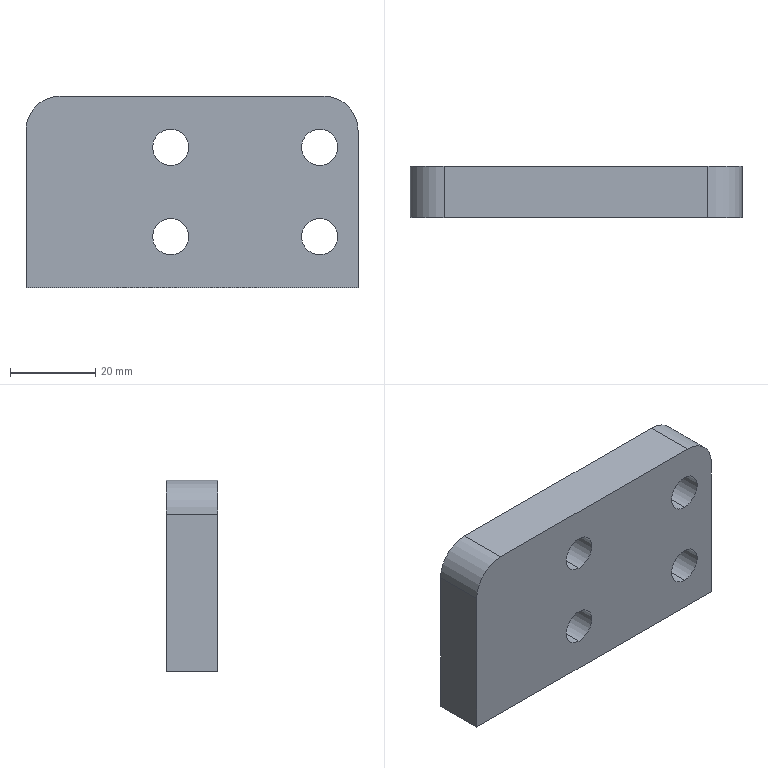Part | SolidWorks | features BaseBody 1 | 1 solid | 36 faces | box 78 x 12 x 45 mm | volume 35458 mm3 | cone 16 | cylinder 14 | plane 6 | commonest cylinder face diameters 8.5 x12 16 x2
STEP:
#1=CARTESIAN_POINT('',(30.,11.225,-14.75));
#2=VERTEX_POINT('',#1);
#3=CARTESIAN_POINT('',(30.,11.225,-6.25));
#4=VERTEX_POINT('',#3);
#5=CARTESIAN_POINT('',(30.,11.225,-10.5));
#6=DIRECTION('',(0.,1.,0.));
#7=DIRECTION('',(0.,0.,1.));
#8=AXIS2_PLACEMENT_3D('',#5,#6,#7);
#9=CIRCLE('',#8,4.25);
#10=EDGE_CURVE('',#2,#4,#9,.T.);
#11=ORIENTED_EDGE('',*,*,#10,.F.);
#12=CARTESIAN_POINT('',(30.,12.,-15.525));
#13=VERTEX_POINT('',#12);
#14=CARTESIAN_POINT('',(30.,12.,-15.525));
#15=DIRECTION('',(0.,0.7071,-0.7071));
#16=VECTOR('',#15,1000.);
#17=LINE('',#14,#16);
#18=EDGE_CURVE('',#2,#13,#17,.T.);
#19=ORIENTED_EDGE('',*,*,#18,.T.);
#20=CARTESIAN_POINT('',(30.,12.,-5.475));
#21=VERTEX_POINT('',#20);
#22=CARTESIAN_POINT('',(30.,12.,-10.5));
#23=DIRECTION('',(0.,1.,0.));
#24=DIRECTION('',(0.,0.,1.));
#25=AXIS2_PLACEMENT_3D('',#22,#23,#24);
#26=CIRCLE('',#25,5.025);
#27=EDGE_CURVE('',#13,#21,#26,.T.);
#28=ORIENTED_EDGE('',*,*,#27,.T.);
#29=CARTESIAN_POINT('',(30.,12.,-5.475));
#30=DIRECTION('',(0.,0.7071,0.7071));
#31=VECTOR('',#30,1000.);
#32=LINE('',#29,#31);
#33=EDGE_CURVE('',#4,#21,#32,.T.);
#34=ORIENTED_EDGE('',*,*,#33,.F.);
#35=EDGE_LOOP('',(#11,#19,#28,#34));
#36=FACE_OUTER_BOUND('',#35,.T.);
#37=CARTESIAN_POINT('',(30.,12.,-10.5));
#38=DIRECTION('',(0.,1.,0.));
#39=DIRECTION('',(0.,0.,1.));
#40=AXIS2_PLACEMENT_3D('',#37,#38,#39);
#41=CONICAL_SURFACE('',#40,5.025,0.7854);
#42=ADVANCED_FACE('',(#36),#41,.F.);
#43=CARTESIAN_POINT('',(30.,0.,-14.75));
#44=VERTEX_POINT('',#43);
#45=CARTESIAN_POINT('',(30.,0.,-6.25));
#46=VERTEX_POINT('',#45);
#47=CARTESIAN_POINT('',(30.,0.,-10.5));
#48=DIRECTION('',(0.,1.,0.));
#49=DIRECTION('',(0.,0.,1.));
#50=AXIS2_PLACEMENT_3D('',#47,#48,#49);
#51=CIRCLE('',#50,4.25);
#52=EDGE_CURVE('',#44,#46,#51,.T.);
#53=ORIENTED_EDGE('',*,*,#52,.F.);
#54=CARTESIAN_POINT('',(30.,12.,-14.75));
#55=DIRECTION('',(0.,1.,0.));
#56=VECTOR('',#55,1000.);
#57=LINE('',#54,#56);
#58=EDGE_CURVE('',#44,#2,#57,.T.);
#59=ORIENTED_EDGE('',*,*,#58,.T.);
#60=ORIENTED_EDGE('',*,*,#10,.T.);
#61=CARTESIAN_POINT('',(30.,12.,-6.25));
#62=DIRECTION('',(0.,1.,0.));
#63=VECTOR('',#62,1000.);
#64=LINE('',#61,#63);
#65=EDGE_CURVE('',#46,#4,#64,.T.);
#66=ORIENTED_EDGE('',*,*,#65,.F.);
#67=EDGE_LOOP('',(#53,#59,#60,#66));
#68=FACE_OUTER_BOUND('',#67,.T.);
#69=CARTESIAN_POINT('',(30.,12.,-10.5));
#70=DIRECTION('',(0.,1.,0.));
#71=DIRECTION('',(0.,0.,1.));
#72=AXIS2_PLACEMENT_3D('',#69,#70,#71);
#73=CYLINDRICAL_SURFACE('',#72,4.25);
#74=ADVANCED_FACE('',(#68),#73,.F.);
#75=CARTESIAN_POINT('',(-5.,11.225,-14.75));
#76=VERTEX_POINT('',#75);
#77=CARTESIAN_POINT('',(-5.,11.225,-6.25));
#78=VERTEX_POINT('',#77);
#79=CARTESIAN_POINT('',(-5.,11.225,-10.5));
#80=DIRECTION('',(0.,1.,0.));
#81=DIRECTION('',(0.,0.,1.));
#82=AXIS2_PLACEMENT_3D('',#79,#80,#81);
#83=CIRCLE('',#82,4.25);
#84=EDGE_CURVE('',#76,#78,#83,.T.);
#85=ORIENTED_EDGE('',*,*,#84,.F.);
#86=CARTESIAN_POINT('',(-5.,12.,-15.525));
#87=VERTEX_POINT('',#86);
#88=CARTESIAN_POINT('',(-5.,12.,-15.525));
#89=DIRECTION('',(0.,0.7071,-0.7071));
#90=VECTOR('',#89,1000.);
#91=LINE('',#88,#90);
#92=EDGE_CURVE('',#76,#87,#91,.T.);
#93=ORIENTED_EDGE('',*,*,#92,.T.);
#94=CARTESIAN_POINT('',(-5.,12.,-5.475));
#95=VERTEX_POINT('',#94);
#96=CARTESIAN_POINT('',(-5.,12.,-10.5));
#97=DIRECTION('',(0.,1.,0.));
#98=DIRECTION('',(0.,0.,1.));
#99=AXIS2_PLACEMENT_3D('',#96,#97,#98);
#100=CIRCLE('',#99,5.025);
#101=EDGE_CURVE('',#87,#95,#100,.T.);
#102=ORIENTED_EDGE('',*,*,#101,.T.);
#103=CARTESIAN_POINT('',(-5.,12.,-5.475));
#104=DIRECTION('',(0.,0.7071,0.7071));
#105=VECTOR('',#104,1000.);
#106=LINE('',#103,#105);
#107=EDGE_CURVE('',#78,#95,#106,.T.);
#108=ORIENTED_EDGE('',*,*,#107,.F.);
#109=EDGE_LOOP('',(#85,#93,#102,#108));
#110=FACE_OUTER_BOUND('',#109,.T.);
#111=CARTESIAN_POINT('',(-5.,12.,-10.5));
#112=DIRECTION('',(0.,1.,0.));
#113=DIRECTION('',(0.,0.,1.));
#114=AXIS2_PLACEMENT_3D('',#111,#112,#113);
#115=CONICAL_SURFACE('',#114,5.025,0.7854);
#116=ADVANCED_FACE('',(#110),#115,.F.);
#117=CARTESIAN_POINT('',(-5.,0.,-14.75));
#118=VERTEX_POINT('',#117);
#119=CARTESIAN_POINT('',(-5.,0.,-6.25));
#120=VERTEX_POINT('',#119);
#121=CARTESIAN_POINT('',(-5.,0.,-10.5));
#122=DIRECTION('',(0.,1.,0.));
#123=DIRECTION('',(0.,0.,1.));
#124=AXIS2_PLACEMENT_3D('',#121,#122,#123);
#125=CIRCLE('',#124,4.25);
#126=EDGE_CURVE('',#118,#120,#125,.T.);
#127=ORIENTED_EDGE('',*,*,#126,.F.);
#128=CARTESIAN_POINT('',(-5.,12.,-14.75));
#129=DIRECTION('',(0.,1.,0.));
#130=VECTOR('',#129,1000.);
#131=LINE('',#128,#130);
#132=EDGE_CURVE('',#118,#76,#131,.T.);
#133=ORIENTED_EDGE('',*,*,#132,.T.);
#134=ORIENTED_EDGE('',*,*,#84,.T.);
#135=CARTESIAN_POINT('',(-5.,12.,-6.25));
#136=DIRECTION('',(0.,1.,0.));
#137=VECTOR('',#136,1000.);
#138=LINE('',#135,#137);
#139=EDGE_CURVE('',#120,#78,#138,.T.);
#140=ORIENTED_EDGE('',*,*,#139,.F.);
#141=EDGE_LOOP('',(#127,#133,#134,#140));
#142=FACE_OUTER_BOUND('',#141,.T.);
#143=CARTESIAN_POINT('',(-5.,12.,-10.5));
#144=DIRECTION('',(0.,1.,0.));
#145=DIRECTION('',(0.,0.,1.));
#146=AXIS2_PLACEMENT_3D('',#143,#144,#145);
#147=CYLINDRICAL_SURFACE('',#146,4.25);
#148=ADVANCED_FACE('',(#142),#147,.F.);
#149=CARTESIAN_POINT('',(-5.,11.225,6.25));
#150=VERTEX_POINT('',#149);
#151=CARTESIAN_POINT('',(-5.,11.225,14.75));
#152=VERTEX_POINT('',#151);
#153=CARTESIAN_POINT('',(-5.,11.225,10.5));
#154=DIRECTION('',(0.,1.,0.));
#155=DIRECTION('',(0.,0.,1.));
#156=AXIS2_PLACEMENT_3D('',#153,#154,#155);
#157=CIRCLE('',#156,4.25);
#158=EDGE_CURVE('',#150,#152,#157,.T.);
#159=ORIENTED_EDGE('',*,*,#158,.F.);
#160=CARTESIAN_POINT('',(-5.,12.,5.475));
#161=VERTEX_POINT('',#160);
#162=CARTESIAN_POINT('',(-5.,12.,5.475));
#163=DIRECTION('',(0.,0.7071,-0.7071));
#164=VECTOR('',#163,1000.);
#165=LINE('',#162,#164);
#166=EDGE_CURVE('',#150,#161,#165,.T.);
#167=ORIENTED_EDGE('',*,*,#166,.T.);
#168=CARTESIAN_POINT('',(-5.,12.,15.525));
#169=VERTEX_POINT('',#168);
#170=CARTESIAN_POINT('',(-5.,12.,10.5));
#171=DIRECTION('',(0.,1.,0.));
#172=DIRECTION('',(0.,0.,1.));
#173=AXIS2_PLACEMENT_3D('',#170,#171,#172);
#174=CIRCLE('',#173,5.025);
#175=EDGE_CURVE('',#161,#169,#174,.T.);
#176=ORIENTED_EDGE('',*,*,#175,.T.);
#177=CARTESIAN_POINT('',(-5.,12.,15.525));
#178=DIRECTION('',(0.,0.7071,0.7071));
#179=VECTOR('',#178,1000.);
#180=LINE('',#177,#179);
#181=EDGE_CURVE('',#152,#169,#180,.T.);
#182=ORIENTED_EDGE('',*,*,#181,.F.);
#183=EDGE_LOOP('',(#159,#167,#176,#182));
#184=FACE_OUTER_BOUND('',#183,.T.);
#185=CARTESIAN_POINT('',(-5.,12.,10.5));
#186=DIRECTION('',(0.,1.,0.));
#187=DIRECTION('',(0.,0.,1.));
#188=AXIS2_PLACEMENT_3D('',#185,#186,#187);
#189=CONICAL_SURFACE('',#188,5.025,0.7854);
#190=ADVANCED_FACE('',(#184),#189,.F.);
#191=CARTESIAN_POINT('',(-5.,0.,6.25));
#192=VERTEX_POINT('',#191);
#193=CARTESIAN_POINT('',(-5.,0.,14.75));
#194=VERTEX_POINT('',#193);
#195=CARTESIAN_POINT('',(-5.,0.,10.5));
#196=DIRECTION('',(0.,1.,0.));
#197=DIRECTION('',(0.,0.,1.));
#198=AXIS2_PLACEMENT_3D('',#195,#196,#197);
#199=CIRCLE('',#198,4.25);
#200=EDGE_CURVE('',#192,#194,#199,.T.);
#201=ORIENTED_EDGE('',*,*,#200,.F.);
#202=CARTESIAN_POINT('',(-5.,12.,6.25));
#203=DIRECTION('',(0.,1.,0.));
#204=VECTOR('',#203,1000.);
#205=LINE('',#202,#204);
#206=EDGE_CURVE('',#192,#150,#205,.T.);
#207=ORIENTED_EDGE('',*,*,#206,.T.);
#208=ORIENTED_EDGE('',*,*,#158,.T.);
#209=CARTESIAN_POINT('',(-5.,12.,14.75));
#210=DIRECTION('',(0.,1.,0.));
#211=VECTOR('',#210,1000.);
#212=LINE('',#209,#211);
#213=EDGE_CURVE('',#194,#152,#212,.T.);
#214=ORIENTED_EDGE('',*,*,#213,.F.);
#215=EDGE_LOOP('',(#201,#207,#208,#214));
#216=FACE_OUTER_BOUND('',#215,.T.);
#217=CARTESIAN_POINT('',(-5.,12.,10.5));
#218=DIRECTION('',(0.,1.,0.));
#219=DIRECTION('',(0.,0.,1.));
#220=AXIS2_PLACEMENT_3D('',#217,#218,#219);
#221=CYLINDRICAL_SURFACE('',#220,4.25);
#222=ADVANCED_FACE('',(#216),#221,.F.);
#223=CARTESIAN_POINT('',(30.,11.225,6.25));
#224=VERTEX_POINT('',#223);
#225=CARTESIAN_POINT('',(30.,11.225,14.75));
#226=VERTEX_POINT('',#225);
#227=CARTESIAN_POINT('',(30.,11.225,10.5));
#228=DIRECTION('',(0.,1.,0.));
#229=DIRECTION('',(0.,0.,1.));
#230=AXIS2_PLACEMENT_3D('',#227,#228,#229);
#231=CIRCLE('',#230,4.25);
#232=EDGE_CURVE('',#224,#226,#231,.T.);
#233=ORIENTED_EDGE('',*,*,#232,.F.);
#234=CARTESIAN_POINT('',(30.,12.,5.475));
#235=VERTEX_POINT('',#234);
#236=CARTESIAN_POINT('',(30.,12.,5.475));
#237=DIRECTION('',(0.,0.7071,-0.7071));
#238=VECTOR('',#237,1000.);
#239=LINE('',#236,#238);
#240=EDGE_CURVE('',#224,#235,#239,.T.);
#241=ORIENTED_EDGE('',*,*,#240,.T.);
#242=CARTESIAN_POINT('',(30.,12.,15.525));
#243=VERTEX_POINT('',#242);
#244=CARTESIAN_POINT('',(30.,12.,10.5));
#245=DIRECTION('',(0.,1.,0.));
#246=DIRECTION('',(0.,0.,1.));
#247=AXIS2_PLACEMENT_3D('',#244,#245,#246);
#248=CIRCLE('',#247,5.025);
#249=EDGE_CURVE('',#235,#243,#248,.T.);
#250=ORIENTED_EDGE('',*,*,#249,.T.);
#251=CARTESIAN_POINT('',(30.,12.,15.525));
#252=DIRECTION('',(0.,0.7071,0.7071));
#253=VECTOR('',#252,1000.);
#254=LINE('',#251,#253);
#255=EDGE_CURVE('',#226,#243,#254,.T.);
#256=ORIENTED_EDGE('',*,*,#255,.F.);
#257=EDGE_LOOP('',(#233,#241,#250,#256));
#258=FACE_OUTER_BOUND('',#257,.T.);
#259=CARTESIAN_POINT('',(30.,12.,10.5));
#260=DIRECTION('',(0.,1.,0.));
#261=DIRECTION('',(0.,0.,1.));
#262=AXIS2_PLACEMENT_3D('',#259,#260,#261);
#263=CONICAL_SURFACE('',#262,5.025,0.7854);
#264=ADVANCED_FACE('',(#258),#263,.F.);
#265=CARTESIAN_POINT('',(30.,0.,6.25));
#266=VERTEX_POINT('',#265);
#267=CARTESIAN_POINT('',(30.,0.,14.75));
#268=VERTEX_POINT('',#267);
#269=CARTESIAN_POINT('',(30.,0.,10.5));
#270=DIRECTION('',(0.,1.,0.));
#271=DIRECTION('',(0.,0.,1.));
#272=AXIS2_PLACEMENT_3D('',#269,#270,#271);
#273=CIRCLE('',#272,4.25);
#274=EDGE_CURVE('',#266,#268,#273,.T.);
#275=ORIENTED_EDGE('',*,*,#274,.F.);
#276=CARTESIAN_POINT('',(30.,12.,6.25));
#277=DIRECTION('',(0.,1.,0.));
#278=VECTOR('',#277,1000.);
#279=LINE('',#276,#278);
#280=EDGE_CURVE('',#266,#224,#279,.T.);
#281=ORIENTED_EDGE('',*,*,#280,.T.);
#282=ORIENTED_EDGE('',*,*,#232,.T.);
#283=CARTESIAN_POINT('',(30.,12.,14.75));
#284=DIRECTION('',(0.,1.,0.));
#285=VECTOR('',#284,1000.);
#286=LINE('',#283,#285);
#287=EDGE_CURVE('',#268,#226,#286,.T.);
#288=ORIENTED_EDGE('',*,*,#287,.F.);
#289=EDGE_LOOP('',(#275,#281,#282,#288));
#290=FACE_OUTER_BOUND('',#289,.T.);
#291=CARTESIAN_POINT('',(30.,12.,10.5));
#292=DIRECTION('',(0.,1.,0.));
#293=DIRECTION('',(0.,0.,1.));
#294=AXIS2_PLACEMENT_3D('',#291,#292,#293);
#295=CYLINDRICAL_SURFACE('',#294,4.25);
#296=ADVANCED_FACE('',(#290),#295,.F.);
#297=CARTESIAN_POINT('',(-22.75,6.,-21.725));
#298=VERTEX_POINT('',#297);
#299=CARTESIAN_POINT('',(-31.25,6.,-21.725));
#300=VERTEX_POINT('',#299);
#301=CARTESIAN_POINT('',(-27.,6.,-21.725));
#302=DIRECTION('',(0.,0.,-1.));
#303=DIRECTION('',(-1.,0.,0.));
#304=AXIS2_PLACEMENT_3D('',#301,#302,#303);
#305=CIRCLE('',#304,4.25);
#306=EDGE_CURVE('',#298,#300,#305,.T.);
#307=ORIENTED_EDGE('',*,*,#306,.F.);
#308=CARTESIAN_POINT('',(-21.975,6.,-22.5));
#309=VERTEX_POINT('',#308);
#310=CARTESIAN_POINT('',(-21.975,6.,-22.5));
#311=DIRECTION('',(0.7071,0.,-0.7071));
#312=VECTOR('',#311,1000.);
#313=LINE('',#310,#312);
#314=EDGE_CURVE('',#298,#309,#313,.T.);
#315=ORIENTED_EDGE('',*,*,#314,.T.);
#316=CARTESIAN_POINT('',(-32.025,6.,-22.5));
#317=VERTEX_POINT('',#316);
#318=CARTESIAN_POINT('',(-27.,6.,-22.5));
#319=DIRECTION('',(0.,0.,-1.));
#320=DIRECTION('',(-1.,0.,0.));
#321=AXIS2_PLACEMENT_3D('',#318,#319,#320);
#322=CIRCLE('',#321,5.025);
#323=EDGE_CURVE('',#309,#317,#322,.T.);
#324=ORIENTED_EDGE('',*,*,#323,.T.);
#325=CARTESIAN_POINT('',(-32.025,6.,-22.5));
#326=DIRECTION('',(-0.7071,0.,-0.7071));
#327=VECTOR('',#326,1000.);
#328=LINE('',#325,#327);
#329=EDGE_CURVE('',#300,#317,#328,.T.);
#330=ORIENTED_EDGE('',*,*,#329,.F.);
#331=EDGE_LOOP('',(#307,#315,#324,#330));
#332=FACE_OUTER_BOUND('',#331,.T.);
#333=CARTESIAN_POINT('',(-27.,6.,-22.5));
#334=DIRECTION('',(0.,0.,-1.));
#335=DIRECTION('',(-1.,0.,0.));
#336=AXIS2_PLACEMENT_3D('',#333,#334,#335);
#337=CONICAL_SURFACE('',#336,5.025,0.7854);
#338=ADVANCED_FACE('',(#332),#337,.F.);
#339=CARTESIAN_POINT('',(-22.75,6.,8.));
#340=VERTEX_POINT('',#339);
#341=CARTESIAN_POINT('',(-31.25,6.,8.));
#342=VERTEX_POINT('',#341);
#343=CARTESIAN_POINT('',(-27.,6.,8.));
#344=DIRECTION('',(0.,0.,-1.));
#345=DIRECTION('',(-1.,0.,0.));
#346=AXIS2_PLACEMENT_3D('',#343,#344,#345);
#347=CIRCLE('',#346,4.25);
#348=EDGE_CURVE('',#340,#342,#347,.T.);
#349=ORIENTED_EDGE('',*,*,#348,.F.);
#350=CARTESIAN_POINT('',(-22.75,6.,-22.5));
#351=DIRECTION('',(0.,0.,-1.));
#352=VECTOR('',#351,1000.);
#353=LINE('',#350,#352);
#354=EDGE_CURVE('',#340,#298,#353,.T.);
#355=ORIENTED_EDGE('',*,*,#354,.T.);
#356=ORIENTED_EDGE('',*,*,#306,.T.);
#357=CARTESIAN_POINT('',(-31.25,6.,-22.5));
#358=DIRECTION('',(0.,0.,-1.));
#359=VECTOR('',#358,1000.);
#360=LINE('',#357,#359);
#361=EDGE_CURVE('',#342,#300,#360,.T.);
#362=ORIENTED_EDGE('',*,*,#361,.F.);
#363=EDGE_LOOP('',(#349,#355,#356,#362));
#364=FACE_OUTER_BOUND('',#363,.T.);
#365=CARTESIAN_POINT('',(-27.,6.,-22.5));
#366=DIRECTION('',(0.,0.,-1.));
#367=DIRECTION('',(-1.,0.,0.));
#368=AXIS2_PLACEMENT_3D('',#365,#366,#367);
#369=CYLINDRICAL_SURFACE('',#368,4.25);
#370=ADVANCED_FACE('',(#364),#369,.F.);
#371=CARTESIAN_POINT('',(-27.,6.,10.554));
#372=VERTEX_POINT('',#371);
#373=CARTESIAN_POINT('',(-31.25,6.,8.));
#374=DIRECTION('',(-0.8572,0.,-0.515));
#375=VECTOR('',#374,1000.);
#376=LINE('',#373,#375);
#377=EDGE_CURVE('',#372,#342,#376,.T.);
#378=ORIENTED_EDGE('',*,*,#377,.F.);
#379=CARTESIAN_POINT('',(-22.75,6.,8.));
#380=DIRECTION('',(0.8572,0.,-0.515));
#381=VECTOR('',#380,1000.);
#382=LINE('',#379,#381);
#383=EDGE_CURVE('',#372,#340,#382,.T.);
#384=ORIENTED_EDGE('',*,*,#383,.T.);
#385=ORIENTED_EDGE('',*,*,#348,.T.);
#386=EDGE_LOOP('',(#378,#384,#385));
#387=FACE_OUTER_BOUND('',#386,.T.);
#388=CARTESIAN_POINT('',(-27.,6.,8.));
#389=DIRECTION('',(0.,0.,-1.));
#390=DIRECTION('',(-1.,0.,0.));
#391=AXIS2_PLACEMENT_3D('',#388,#389,#390);
#392=CONICAL_SURFACE('',#391,4.25,1.03);
#393=ADVANCED_FACE('',(#387),#392,.F.);
#394=CARTESIAN_POINT('',(21.25,6.,-21.725));
#395=VERTEX_POINT('',#394);
#396=CARTESIAN_POINT('',(12.75,6.,-21.725));
#397=VERTEX_POINT('',#396);
#398=CARTESIAN_POINT('',(17.,6.,-21.725));
#399=DIRECTION('',(0.,0.,-1.));
#400=DIRECTION('',(-1.,0.,0.));
#401=AXIS2_PLACEMENT_3D('',#398,#399,#400);
#402=CIRCLE('',#401,4.25);
#403=EDGE_CURVE('',#395,#397,#402,.T.);
#404=ORIENTED_EDGE('',*,*,#403,.F.);
#405=CARTESIAN_POINT('',(22.025,6.,-22.5));
#406=VERTEX_POINT('',#405);
#407=CARTESIAN_POINT('',(22.025,6.,-22.5));
#408=DIRECTION('',(0.7071,0.,-0.7071));
#409=VECTOR('',#408,1000.);
#410=LINE('',#407,#409);
#411=EDGE_CURVE('',#395,#406,#410,.T.);
#412=ORIENTED_EDGE('',*,*,#411,.T.);
#413=CARTESIAN_POINT('',(11.975,6.,-22.5));
#414=VERTEX_POINT('',#413);
#415=CARTESIAN_POINT('',(17.,6.,-22.5));
#416=DIRECTION('',(0.,0.,-1.));
#417=DIRECTION('',(-1.,0.,0.));
#418=AXIS2_PLACEMENT_3D('',#415,#416,#417);
#419=CIRCLE('',#418,5.025);
#420=EDGE_CURVE('',#406,#414,#419,.T.);
#421=ORIENTED_EDGE('',*,*,#420,.T.);
#422=CARTESIAN_POINT('',(11.975,6.,-22.5));
#423=DIRECTION('',(-0.7071,0.,-0.7071));
#424=VECTOR('',#423,1000.);
#425=LINE('',#422,#424);
#426=EDGE_CURVE('',#397,#414,#425,.T.);
#427=ORIENTED_EDGE('',*,*,#426,.F.);
#428=EDGE_LOOP('',(#404,#412,#421,#427));
#429=FACE_OUTER_BOUND('',#428,.T.);
#430=CARTESIAN_POINT('',(17.,6.,-22.5));
#431=DIRECTION('',(0.,0.,-1.));
#432=DIRECTION('',(-1.,0.,0.));
#433=AXIS2_PLACEMENT_3D('',#430,#431,#432);
#434=CONICAL_SURFACE('',#433,5.025,0.7854);
#435=ADVANCED_FACE('',(#429),#434,.F.);
#436=CARTESIAN_POINT('',(21.25,6.,8.));
#437=VERTEX_POINT('',#436);
#438=CARTESIAN_POINT('',(12.75,6.,8.));
#439=VERTEX_POINT('',#438);
#440=CARTESIAN_POINT('',(17.,6.,8.));
#441=DIRECTION('',(0.,0.,-1.));
#442=DIRECTION('',(-1.,0.,0.));
#443=AXIS2_PLACEMENT_3D('',#440,#441,#442);
#444=CIRCLE('',#443,4.25);
#445=EDGE_CURVE('',#437,#439,#444,.T.);
#446=ORIENTED_EDGE('',*,*,#445,.F.);
#447=CARTESIAN_POINT('',(21.25,6.,-22.5));
#448=DIRECTION('',(0.,0.,-1.));
#449=VECTOR('',#448,1000.);
#450=LINE('',#447,#449);
#451=EDGE_CURVE('',#437,#395,#450,.T.);
#452=ORIENTED_EDGE('',*,*,#451,.T.);
#453=ORIENTED_EDGE('',*,*,#403,.T.);
#454=CARTESIAN_POINT('',(12.75,6.,-22.5));
#455=DIRECTION('',(0.,0.,-1.));
#456=VECTOR('',#455,1000.);
#457=LINE('',#454,#456);
#458=EDGE_CURVE('',#439,#397,#457,.T.);
#459=ORIENTED_EDGE('',*,*,#458,.F.);
#460=EDGE_LOOP('',(#446,#452,#453,#459));
#461=FACE_OUTER_BOUND('',#460,.T.);
#462=CARTESIAN_POINT('',(17.,6.,-22.5));
#463=DIRECTION('',(0.,0.,-1.));
#464=DIRECTION('',(-1.,0.,0.));
#465=AXIS2_PLACEMENT_3D('',#462,#463,#464);
#466=CYLINDRICAL_SURFACE('',#465,4.25);
#467=ADVANCED_FACE('',(#461),#466,.F.);
#468=CARTESIAN_POINT('',(17.,6.,10.554));
#469=VERTEX_POINT('',#468);
#470=CARTESIAN_POINT('',(12.75,6.,8.));
#471=DIRECTION('',(-0.8572,0.,-0.515));
#472=VECTOR('',#471,1000.);
#473=LINE('',#470,#472);
#474=EDGE_CURVE('',#469,#439,#473,.T.);
#475=ORIENTED_EDGE('',*,*,#474,.F.);
#476=CARTESIAN_POINT('',(21.25,6.,8.));
#477=DIRECTION('',(0.8572,0.,-0.515));
#478=VECTOR('',#477,1000.);
#479=LINE('',#476,#478);
#480=EDGE_CURVE('',#469,#437,#479,.T.);
#481=ORIENTED_EDGE('',*,*,#480,.T.);
#482=ORIENTED_EDGE('',*,*,#445,.T.);
#483=EDGE_LOOP('',(#475,#481,#482));
#484=FACE_OUTER_BOUND('',#483,.T.);
#485=CARTESIAN_POINT('',(17.,6.,8.));
#486=DIRECTION('',(0.,0.,-1.));
#487=DIRECTION('',(-1.,0.,0.));
#488=AXIS2_PLACEMENT_3D('',#485,#486,#487);
#489=CONICAL_SURFACE('',#488,4.25,1.03);
#490=ADVANCED_FACE('',(#484),#489,.F.);
#491=CARTESIAN_POINT('',(39.,12.,14.5));
#492=VERTEX_POINT('',#491);
#493=CARTESIAN_POINT('',(39.,12.,-22.5));
#494=VERTEX_POINT('',#493);
#495=CARTESIAN_POINT('',(39.,12.,-22.5));
#496=DIRECTION('',(0.,0.,-1.));
#497=VECTOR('',#496,1000.);
#498=LINE('',#495,#497);
#499=EDGE_CURVE('',#492,#494,#498,.T.);
#500=ORIENTED_EDGE('',*,*,#499,.F.);
#501=CARTESIAN_POINT('',(39.,0.,14.5));
#502=VERTEX_POINT('',#501);
#503=CARTESIAN_POINT('',(39.,12.,14.5));
#504=DIRECTION('',(0.,-1.,0.));
#505=VECTOR('',#504,1000.);
#506=LINE('',#503,#505);
#507=EDGE_CURVE('',#492,#502,#506,.T.);
#508=ORIENTED_EDGE('',*,*,#507,.T.);
#509=CARTESIAN_POINT('',(39.,0.,-22.5));
#510=VERTEX_POINT('',#509);
#511=CARTESIAN_POINT('',(39.,0.,-22.5));
#512=DIRECTION('',(0.,0.,-1.));
#513=VECTOR('',#512,1000.);
#514=LINE('',#511,#513);
#515=EDGE_CURVE('',#502,#510,#514,.T.);
#516=ORIENTED_EDGE('',*,*,#515,.T.);
#517=CARTESIAN_POINT('',(39.,12.,-22.5));
#518=DIRECTION('',(0.,-1.,0.));
#519=VECTOR('',#518,1000.);
#520=LINE('',#517,#519);
#521=EDGE_CURVE('',#494,#510,#520,.T.);
#522=ORIENTED_EDGE('',*,*,#521,.F.);
#523=EDGE_LOOP('',(#500,#508,#516,#522));
#524=FACE_OUTER_BOUND('',#523,.T.);
#525=CARTESIAN_POINT('',(39.,12.,-22.5));
#526=DIRECTION('',(-1.,0.,0.));
#527=DIRECTION('',(0.,0.,1.));
#528=AXIS2_PLACEMENT_3D('',#525,#526,#527);
#529=PLANE('',#528);
#530=ADVANCED_FACE('',(#524),#529,.F.);
#531=CARTESIAN_POINT('',(-27.,6.,-22.5));
#532=DIRECTION('',(0.,0.,-1.));
#533=DIRECTION('',(-1.,0.,0.));
#534=AXIS2_PLACEMENT_3D('',#531,#532,#533);
#535=CIRCLE('',#534,5.025);
#536=EDGE_CURVE('',#317,#309,#535,.T.);
#537=ORIENTED_EDGE('',*,*,#536,.F.);
#538=ORIENTED_EDGE('',*,*,#323,.F.);
#539=EDGE_LOOP('',(#537,#538));
#540=FACE_BOUND('',#539,.T.);
#541=CARTESIAN_POINT('',(17.,6.,-22.5));
#542=DIRECTION('',(0.,0.,-1.));
#543=DIRECTION('',(-1.,0.,0.));
#544=AXIS2_PLACEMENT_3D('',#541,#542,#543);
#545=CIRCLE('',#544,5.025);
#546=EDGE_CURVE('',#414,#406,#545,.T.);
#547=ORIENTED_EDGE('',*,*,#546,.F.);
#548=ORIENTED_EDGE('',*,*,#420,.F.);
#549=EDGE_LOOP('',(#547,#548));
#550=FACE_BOUND('',#549,.T.);
#551=CARTESIAN_POINT('',(-39.,0.,-22.5));
#552=VERTEX_POINT('',#551);
#553=CARTESIAN_POINT('',(-39.,0.,-22.5));
#554=DIRECTION('',(-1.,0.,0.));
#555=VECTOR('',#554,1000.);
#556=LINE('',#553,#555);
#557=EDGE_CURVE('',#510,#552,#556,.T.);
#558=ORIENTED_EDGE('',*,*,#557,.T.);
#559=CARTESIAN_POINT('',(-39.,12.,-22.5));
#560=VERTEX_POINT('',#559);
#561=CARTESIAN_POINT('',(-39.,12.,-22.5));
#562=DIRECTION('',(0.,-1.,0.));
#563=VECTOR('',#562,1000.);
#564=LINE('',#561,#563);
#565=EDGE_CURVE('',#560,#552,#564,.T.);
#566=ORIENTED_EDGE('',*,*,#565,.F.);
#567=CARTESIAN_POINT('',(-39.,12.,-22.5));
#568=DIRECTION('',(-1.,0.,0.));
#569=VECTOR('',#568,1000.);
#570=LINE('',#567,#569);
#571=EDGE_CURVE('',#494,#560,#570,.T.);
#572=ORIENTED_EDGE('',*,*,#571,.F.);
#573=ORIENTED_EDGE('',*,*,#521,.T.);
#574=EDGE_LOOP('',(#558,#566,#572,#573));
#575=FACE_OUTER_BOUND('',#574,.T.);
#576=CARTESIAN_POINT('',(-39.,12.,-22.5));
#577=DIRECTION('',(0.,0.,1.));
#578=DIRECTION('',(1.,0.,0.));
#579=AXIS2_PLACEMENT_3D('',#576,#577,#578);
#580=PLANE('',#579);
#581=ADVANCED_FACE('',(#540,#550,#575),#580,.F.);
#582=CARTESIAN_POINT('',(-39.,0.,14.5));
#583=VERTEX_POINT('',#582);
#584=CARTESIAN_POINT('',(-39.,0.,-22.5));
#585=DIRECTION('',(0.,0.,1.));
#586=VECTOR('',#585,1000.);
#587=LINE('',#584,#586);
#588=EDGE_CURVE('',#552,#583,#587,.T.);
#589=ORIENTED_EDGE('',*,*,#588,.T.);
#590=CARTESIAN_POINT('',(-39.,12.,14.5));
#591=VERTEX_POINT('',#590);
#592=CARTESIAN_POINT('',(-39.,12.,14.5));
#593=DIRECTION('',(0.,1.,0.));
#594=VECTOR('',#593,1000.);
#595=LINE('',#592,#594);
#596=EDGE_CURVE('',#583,#591,#595,.T.);
#597=ORIENTED_EDGE('',*,*,#596,.T.);
#598=CARTESIAN_POINT('',(-39.,12.,-22.5));
#599=DIRECTION('',(0.,0.,1.));
#600=VECTOR('',#599,1000.);
#601=LINE('',#598,#600);
#602=EDGE_CURVE('',#560,#591,#601,.T.);
#603=ORIENTED_EDGE('',*,*,#602,.F.);
#604=ORIENTED_EDGE('',*,*,#565,.T.);
#605=EDGE_LOOP('',(#589,#597,#603,#604));
#606=FACE_OUTER_BOUND('',#605,.T.);
#607=CARTESIAN_POINT('',(-39.,12.,-22.5));
#608=DIRECTION('',(1.,0.,0.));
#609=DIRECTION('',(0.,0.,-1.));
#610=AXIS2_PLACEMENT_3D('',#607,#608,#609);
#611=PLANE('',#610);
#612=ADVANCED_FACE('',(#606),#611,.F.);
#613=CARTESIAN_POINT('',(-31.,0.,22.5));
#614=VERTEX_POINT('',#613);
#615=CARTESIAN_POINT('',(31.,0.,22.5));
#616=VERTEX_POINT('',#615);
#617=CARTESIAN_POINT('',(-39.,0.,22.5));
#618=DIRECTION('',(1.,0.,0.));
#619=VECTOR('',#618,1000.);
#620=LINE('',#617,#619);
#621=EDGE_CURVE('',#614,#616,#620,.T.);
#622=ORIENTED_EDGE('',*,*,#621,.T.);
#623=CARTESIAN_POINT('',(31.,12.,22.5));
#624=VERTEX_POINT('',#623);
#625=CARTESIAN_POINT('',(31.,12.,22.5));
#626=DIRECTION('',(0.,1.,0.));
#627=VECTOR('',#626,1000.);
#628=LINE('',#625,#627);
#629=EDGE_CURVE('',#616,#624,#628,.T.);
#630=ORIENTED_EDGE('',*,*,#629,.T.);
#631=CARTESIAN_POINT('',(-31.,12.,22.5));
#632=VERTEX_POINT('',#631);
#633=CARTESIAN_POINT('',(-39.,12.,22.5));
#634=DIRECTION('',(1.,0.,0.));
#635=VECTOR('',#634,1000.);
#636=LINE('',#633,#635);
#637=EDGE_CURVE('',#632,#624,#636,.T.);
#638=ORIENTED_EDGE('',*,*,#637,.F.);
#639=CARTESIAN_POINT('',(-31.,12.,22.5));
#640=DIRECTION('',(0.,-1.,0.));
#641=VECTOR('',#640,1000.);
#642=LINE('',#639,#641);
#643=EDGE_CURVE('',#632,#614,#642,.T.);
#644=ORIENTED_EDGE('',*,*,#643,.T.);
#645=EDGE_LOOP('',(#622,#630,#638,#644));
#646=FACE_OUTER_BOUND('',#645,.T.);
#647=CARTESIAN_POINT('',(-39.,12.,22.5));
#648=DIRECTION('',(0.,0.,-1.));
#649=DIRECTION('',(-1.,0.,0.));
#650=AXIS2_PLACEMENT_3D('',#647,#648,#649);
#651=PLANE('',#650);
#652=ADVANCED_FACE('',(#646),#651,.F.);
#653=CARTESIAN_POINT('',(30.,12.,-10.5));
#654=DIRECTION('',(0.,1.,0.));
#655=DIRECTION('',(0.,0.,1.));
#656=AXIS2_PLACEMENT_3D('',#653,#654,#655);
#657=CIRCLE('',#656,5.025);
#658=EDGE_CURVE('',#21,#13,#657,.T.);
#659=ORIENTED_EDGE('',*,*,#658,.F.);
#660=ORIENTED_EDGE('',*,*,#27,.F.);
#661=EDGE_LOOP('',(#659,#660));
#662=FACE_BOUND('',#661,.T.);
#663=CARTESIAN_POINT('',(-5.,12.,-10.5));
#664=DIRECTION('',(0.,1.,0.));
#665=DIRECTION('',(0.,0.,1.));
#666=AXIS2_PLACEMENT_3D('',#663,#664,#665);
#667=CIRCLE('',#666,5.025);
#668=EDGE_CURVE('',#95,#87,#667,.T.);
#669=ORIENTED_EDGE('',*,*,#668,.F.);
#670=ORIENTED_EDGE('',*,*,#101,.F.);
#671=EDGE_LOOP('',(#669,#670));
#672=FACE_BOUND('',#671,.T.);
#673=CARTESIAN_POINT('',(-5.,12.,10.5));
#674=DIRECTION('',(0.,1.,0.));
#675=DIRECTION('',(0.,0.,1.));
#676=AXIS2_PLACEMENT_3D('',#673,#674,#675);
#677=CIRCLE('',#676,5.025);
#678=EDGE_CURVE('',#169,#161,#677,.T.);
#679=ORIENTED_EDGE('',*,*,#678,.F.);
#680=ORIENTED_EDGE('',*,*,#175,.F.);
#681=EDGE_LOOP('',(#679,#680));
#682=FACE_BOUND('',#681,.T.);
#683=CARTESIAN_POINT('',(30.,12.,10.5));
#684=DIRECTION('',(0.,1.,0.));
#685=DIRECTION('',(0.,0.,1.));
#686=AXIS2_PLACEMENT_3D('',#683,#684,#685);
#687=CIRCLE('',#686,5.025);
#688=EDGE_CURVE('',#243,#235,#687,.T.);
#689=ORIENTED_EDGE('',*,*,#688,.F.);
#690=ORIENTED_EDGE('',*,*,#249,.F.);
#691=EDGE_LOOP('',(#689,#690));
#692=FACE_BOUND('',#691,.T.);
#693=ORIENTED_EDGE('',*,*,#637,.T.);
#694=CARTESIAN_POINT('',(31.,12.,14.5));
#695=DIRECTION('',(0.,1.,0.));
#696=DIRECTION('',(0.,0.,1.));
#697=AXIS2_PLACEMENT_3D('',#694,#695,#696);
#698=CIRCLE('',#697,8.);
#699=EDGE_CURVE('',#624,#492,#698,.T.);
#700=ORIENTED_EDGE('',*,*,#699,.T.);
#701=ORIENTED_EDGE('',*,*,#499,.T.);
#702=ORIENTED_EDGE('',*,*,#571,.T.);
#703=ORIENTED_EDGE('',*,*,#602,.T.);
#704=CARTESIAN_POINT('',(-31.,12.,14.5));
#705=DIRECTION('',(0.,1.,0.));
#706=DIRECTION('',(0.,0.,1.));
#707=AXIS2_PLACEMENT_3D('',#704,#705,#706);
#708=CIRCLE('',#707,8.);
#709=EDGE_CURVE('',#591,#632,#708,.T.);
#710=ORIENTED_EDGE('',*,*,#709,.T.);
#711=EDGE_LOOP('',(#693,#700,#701,#702,#703,#710));
#712=FACE_OUTER_BOUND('',#711,.T.);
#713=CARTESIAN_POINT('',(0.,12.,0.));
#714=DIRECTION('',(0.,1.,0.));
#715=DIRECTION('',(0.,0.,1.));
#716=AXIS2_PLACEMENT_3D('',#713,#714,#715);
#717=PLANE('',#716);
#718=ADVANCED_FACE('',(#662,#672,#682,#692,#712),#717,.T.);
#719=CARTESIAN_POINT('',(30.,0.,-10.5));
#720=DIRECTION('',(0.,1.,0.));
#721=DIRECTION('',(0.,0.,1.));
#722=AXIS2_PLACEMENT_3D('',#719,#720,#721);
#723=CIRCLE('',#722,4.25);
#724=EDGE_CURVE('',#46,#44,#723,.T.);
#725=ORIENTED_EDGE('',*,*,#724,.T.);
#726=ORIENTED_EDGE('',*,*,#52,.T.);
#727=EDGE_LOOP('',(#725,#726));
#728=FACE_BOUND('',#727,.T.);
#729=CARTESIAN_POINT('',(-5.,0.,-10.5));
#730=DIRECTION('',(0.,1.,0.));
#731=DIRECTION('',(0.,0.,1.));
#732=AXIS2_PLACEMENT_3D('',#729,#730,#731);
#733=CIRCLE('',#732,4.25);
#734=EDGE_CURVE('',#120,#118,#733,.T.);
#735=ORIENTED_EDGE('',*,*,#734,.T.);
#736=ORIENTED_EDGE('',*,*,#126,.T.);
#737=EDGE_LOOP('',(#735,#736));
#738=FACE_BOUND('',#737,.T.);
#739=CARTESIAN_POINT('',(-5.,0.,10.5));
#740=DIRECTION('',(0.,1.,0.));
#741=DIRECTION('',(0.,0.,1.));
#742=AXIS2_PLACEMENT_3D('',#739,#740,#741);
#743=CIRCLE('',#742,4.25);
#744=EDGE_CURVE('',#194,#192,#743,.T.);
#745=ORIENTED_EDGE('',*,*,#744,.T.);
#746=ORIENTED_EDGE('',*,*,#200,.T.);
#747=EDGE_LOOP('',(#745,#746));
#748=FACE_BOUND('',#747,.T.);
#749=CARTESIAN_POINT('',(30.,0.,10.5));
#750=DIRECTION('',(0.,1.,0.));
#751=DIRECTION('',(0.,0.,1.));
#752=AXIS2_PLACEMENT_3D('',#749,#750,#751);
#753=CIRCLE('',#752,4.25);
#754=EDGE_CURVE('',#268,#266,#753,.T.);
#755=ORIENTED_EDGE('',*,*,#754,.T.);
#756=ORIENTED_EDGE('',*,*,#274,.T.);
#757=EDGE_LOOP('',(#755,#756));
#758=FACE_BOUND('',#757,.T.);
#759=ORIENTED_EDGE('',*,*,#515,.F.);
#760=CARTESIAN_POINT('',(31.,0.,14.5));
#761=DIRECTION('',(0.,-1.,0.));
#762=DIRECTION('',(0.,0.,1.));
#763=AXIS2_PLACEMENT_3D('',#760,#761,#762);
#764=CIRCLE('',#763,8.);
#765=EDGE_CURVE('',#502,#616,#764,.T.);
#766=ORIENTED_EDGE('',*,*,#765,.T.);
#767=ORIENTED_EDGE('',*,*,#621,.F.);
#768=CARTESIAN_POINT('',(-31.,0.,14.5));
#769=DIRECTION('',(0.,-1.,0.));
#770=DIRECTION('',(0.,0.,1.));
#771=AXIS2_PLACEMENT_3D('',#768,#769,#770);
#772=CIRCLE('',#771,8.);
#773=EDGE_CURVE('',#614,#583,#772,.T.);
#774=ORIENTED_EDGE('',*,*,#773,.T.);
#775=ORIENTED_EDGE('',*,*,#588,.F.);
#776=ORIENTED_EDGE('',*,*,#557,.F.);
#777=EDGE_LOOP('',(#759,#766,#767,#774,#775,#776));
#778=FACE_OUTER_BOUND('',#777,.T.);
#779=CARTESIAN_POINT('',(0.,0.,0.));
#780=DIRECTION('',(0.,1.,0.));
#781=DIRECTION('',(0.,0.,1.));
#782=AXIS2_PLACEMENT_3D('',#779,#780,#781);
#783=PLANE('',#782);
#784=ADVANCED_FACE('',(#728,#738,#748,#758,#778),#783,.F.);
#785=ORIENTED_EDGE('',*,*,#699,.F.);
#786=ORIENTED_EDGE('',*,*,#629,.F.);
#787=ORIENTED_EDGE('',*,*,#765,.F.);
#788=ORIENTED_EDGE('',*,*,#507,.F.);
#789=EDGE_LOOP('',(#785,#786,#787,#788));
#790=FACE_OUTER_BOUND('',#789,.T.);
#791=CARTESIAN_POINT('',(31.,12.,14.5));
#792=DIRECTION('',(0.,-1.,0.));
#793=DIRECTION('',(0.,0.,-1.));
#794=AXIS2_PLACEMENT_3D('',#791,#792,#793);
#795=CYLINDRICAL_SURFACE('',#794,8.);
#796=ADVANCED_FACE('',(#790),#795,.T.);
#797=ORIENTED_EDGE('',*,*,#709,.F.);
#798=ORIENTED_EDGE('',*,*,#596,.F.);
#799=ORIENTED_EDGE('',*,*,#773,.F.);
#800=ORIENTED_EDGE('',*,*,#643,.F.);
#801=EDGE_LOOP('',(#797,#798,#799,#800));
#802=FACE_OUTER_BOUND('',#801,.T.);
#803=CARTESIAN_POINT('',(-31.,12.,14.5));
#804=DIRECTION('',(0.,-1.,0.));
#805=DIRECTION('',(0.,0.,-1.));
#806=AXIS2_PLACEMENT_3D('',#803,#804,#805);
#807=CYLINDRICAL_SURFACE('',#806,8.);
#808=ADVANCED_FACE('',(#802),#807,.T.);
#809=ORIENTED_EDGE('',*,*,#480,.F.);
#810=ORIENTED_EDGE('',*,*,#474,.T.);
#811=CARTESIAN_POINT('',(17.,6.,8.));
#812=DIRECTION('',(0.,0.,-1.));
#813=DIRECTION('',(-1.,0.,0.));
#814=AXIS2_PLACEMENT_3D('',#811,#812,#813);
#815=CIRCLE('',#814,4.25);
#816=EDGE_CURVE('',#439,#437,#815,.T.);
#817=ORIENTED_EDGE('',*,*,#816,.T.);
#818=EDGE_LOOP('',(#809,#810,#817));
#819=FACE_OUTER_BOUND('',#818,.T.);
#820=CARTESIAN_POINT('',(17.,6.,8.));
#821=DIRECTION('',(0.,0.,-1.));
#822=DIRECTION('',(-1.,0.,0.));
#823=AXIS2_PLACEMENT_3D('',#820,#821,#822);
#824=CONICAL_SURFACE('',#823,4.25,1.03);
#825=ADVANCED_FACE('',(#819),#824,.F.);
#826=ORIENTED_EDGE('',*,*,#451,.F.);
#827=ORIENTED_EDGE('',*,*,#816,.F.);
#828=ORIENTED_EDGE('',*,*,#458,.T.);
#829=CARTESIAN_POINT('',(17.,6.,-21.725));
#830=DIRECTION('',(0.,0.,-1.));
#831=DIRECTION('',(-1.,0.,0.));
#832=AXIS2_PLACEMENT_3D('',#829,#830,#831);
#833=CIRCLE('',#832,4.25);
#834=EDGE_CURVE('',#397,#395,#833,.T.);
#835=ORIENTED_EDGE('',*,*,#834,.T.);
#836=EDGE_LOOP('',(#826,#827,#828,#835));
#837=FACE_OUTER_BOUND('',#836,.T.);
#838=CARTESIAN_POINT('',(17.,6.,-22.5));
#839=DIRECTION('',(0.,0.,-1.));
#840=DIRECTION('',(-1.,0.,0.));
#841=AXIS2_PLACEMENT_3D('',#838,#839,#840);
#842=CYLINDRICAL_SURFACE('',#841,4.25);
#843=ADVANCED_FACE('',(#837),#842,.F.);
#844=ORIENTED_EDGE('',*,*,#411,.F.);
#845=ORIENTED_EDGE('',*,*,#834,.F.);
#846=ORIENTED_EDGE('',*,*,#426,.T.);
#847=ORIENTED_EDGE('',*,*,#546,.T.);
#848=EDGE_LOOP('',(#844,#845,#846,#847));
#849=FACE_OUTER_BOUND('',#848,.T.);
#850=CARTESIAN_POINT('',(17.,6.,-22.5));
#851=DIRECTION('',(0.,0.,-1.));
#852=DIRECTION('',(-1.,0.,0.));
#853=AXIS2_PLACEMENT_3D('',#850,#851,#852);
#854=CONICAL_SURFACE('',#853,5.025,0.7854);
#855=ADVANCED_FACE('',(#849),#854,.F.);
#856=ORIENTED_EDGE('',*,*,#383,.F.);
#857=ORIENTED_EDGE('',*,*,#377,.T.);
#858=CARTESIAN_POINT('',(-27.,6.,8.));
#859=DIRECTION('',(0.,0.,-1.));
#860=DIRECTION('',(-1.,0.,0.));
#861=AXIS2_PLACEMENT_3D('',#858,#859,#860);
#862=CIRCLE('',#861,4.25);
#863=EDGE_CURVE('',#342,#340,#862,.T.);
#864=ORIENTED_EDGE('',*,*,#863,.T.);
#865=EDGE_LOOP('',(#856,#857,#864));
#866=FACE_OUTER_BOUND('',#865,.T.);
#867=CARTESIAN_POINT('',(-27.,6.,8.));
#868=DIRECTION('',(0.,0.,-1.));
#869=DIRECTION('',(-1.,0.,0.));
#870=AXIS2_PLACEMENT_3D('',#867,#868,#869);
#871=CONICAL_SURFACE('',#870,4.25,1.03);
#872=ADVANCED_FACE('',(#866),#871,.F.);
#873=ORIENTED_EDGE('',*,*,#354,.F.);
#874=ORIENTED_EDGE('',*,*,#863,.F.);
#875=ORIENTED_EDGE('',*,*,#361,.T.);
#876=CARTESIAN_POINT('',(-27.,6.,-21.725));
#877=DIRECTION('',(0.,0.,-1.));
#878=DIRECTION('',(-1.,0.,0.));
#879=AXIS2_PLACEMENT_3D('',#876,#877,#878);
#880=CIRCLE('',#879,4.25);
#881=EDGE_CURVE('',#300,#298,#880,.T.);
#882=ORIENTED_EDGE('',*,*,#881,.T.);
#883=EDGE_LOOP('',(#873,#874,#875,#882));
#884=FACE_OUTER_BOUND('',#883,.T.);
#885=CARTESIAN_POINT('',(-27.,6.,-22.5));
#886=DIRECTION('',(0.,0.,-1.));
#887=DIRECTION('',(-1.,0.,0.));
#888=AXIS2_PLACEMENT_3D('',#885,#886,#887);
#889=CYLINDRICAL_SURFACE('',#888,4.25);
#890=ADVANCED_FACE('',(#884),#889,.F.);
#891=ORIENTED_EDGE('',*,*,#314,.F.);
#892=ORIENTED_EDGE('',*,*,#881,.F.);
#893=ORIENTED_EDGE('',*,*,#329,.T.);
#894=ORIENTED_EDGE('',*,*,#536,.T.);
#895=EDGE_LOOP('',(#891,#892,#893,#894));
#896=FACE_OUTER_BOUND('',#895,.T.);
#897=CARTESIAN_POINT('',(-27.,6.,-22.5));
#898=DIRECTION('',(0.,0.,-1.));
#899=DIRECTION('',(-1.,0.,0.));
#900=AXIS2_PLACEMENT_3D('',#897,#898,#899);
#901=CONICAL_SURFACE('',#900,5.025,0.7854);
#902=ADVANCED_FACE('',(#896),#901,.F.);
#903=ORIENTED_EDGE('',*,*,#280,.F.);
#904=ORIENTED_EDGE('',*,*,#754,.F.);
#905=ORIENTED_EDGE('',*,*,#287,.T.);
#906=CARTESIAN_POINT('',(30.,11.225,10.5));
#907=DIRECTION('',(0.,1.,0.));
#908=DIRECTION('',(0.,0.,1.));
#909=AXIS2_PLACEMENT_3D('',#906,#907,#908);
#910=CIRCLE('',#909,4.25);
#911=EDGE_CURVE('',#226,#224,#910,.T.);
#912=ORIENTED_EDGE('',*,*,#911,.T.);
#913=EDGE_LOOP('',(#903,#904,#905,#912));
#914=FACE_OUTER_BOUND('',#913,.T.);
#915=CARTESIAN_POINT('',(30.,12.,10.5));
#916=DIRECTION('',(0.,1.,0.));
#917=DIRECTION('',(0.,0.,1.));
#918=AXIS2_PLACEMENT_3D('',#915,#916,#917);
#919=CYLINDRICAL_SURFACE('',#918,4.25);
#920=ADVANCED_FACE('',(#914),#919,.F.);
#921=ORIENTED_EDGE('',*,*,#240,.F.);
#922=ORIENTED_EDGE('',*,*,#911,.F.);
#923=ORIENTED_EDGE('',*,*,#255,.T.);
#924=ORIENTED_EDGE('',*,*,#688,.T.);
#925=EDGE_LOOP('',(#921,#922,#923,#924));
#926=FACE_OUTER_BOUND('',#925,.T.);
#927=CARTESIAN_POINT('',(30.,12.,10.5));
#928=DIRECTION('',(0.,1.,0.));
#929=DIRECTION('',(0.,0.,1.));
#930=AXIS2_PLACEMENT_3D('',#927,#928,#929);
#931=CONICAL_SURFACE('',#930,5.025,0.7854);
#932=ADVANCED_FACE('',(#926),#931,.F.);
#933=ORIENTED_EDGE('',*,*,#206,.F.);
#934=ORIENTED_EDGE('',*,*,#744,.F.);
#935=ORIENTED_EDGE('',*,*,#213,.T.);
#936=CARTESIAN_POINT('',(-5.,11.225,10.5));
#937=DIRECTION('',(0.,1.,0.));
#938=DIRECTION('',(0.,0.,1.));
#939=AXIS2_PLACEMENT_3D('',#936,#937,#938);
#940=CIRCLE('',#939,4.25);
#941=EDGE_CURVE('',#152,#150,#940,.T.);
#942=ORIENTED_EDGE('',*,*,#941,.T.);
#943=EDGE_LOOP('',(#933,#934,#935,#942));
#944=FACE_OUTER_BOUND('',#943,.T.);
#945=CARTESIAN_POINT('',(-5.,12.,10.5));
#946=DIRECTION('',(0.,1.,0.));
#947=DIRECTION('',(0.,0.,1.));
#948=AXIS2_PLACEMENT_3D('',#945,#946,#947);
#949=CYLINDRICAL_SURFACE('',#948,4.25);
#950=ADVANCED_FACE('',(#944),#949,.F.);
#951=ORIENTED_EDGE('',*,*,#166,.F.);
#952=ORIENTED_EDGE('',*,*,#941,.F.);
#953=ORIENTED_EDGE('',*,*,#181,.T.);
#954=ORIENTED_EDGE('',*,*,#678,.T.);
#955=EDGE_LOOP('',(#951,#952,#953,#954));
#956=FACE_OUTER_BOUND('',#955,.T.);
#957=CARTESIAN_POINT('',(-5.,12.,10.5));
#958=DIRECTION('',(0.,1.,0.));
#959=DIRECTION('',(0.,0.,1.));
#960=AXIS2_PLACEMENT_3D('',#957,#958,#959);
#961=CONICAL_SURFACE('',#960,5.025,0.7854);
#962=ADVANCED_FACE('',(#956),#961,.F.);
#963=ORIENTED_EDGE('',*,*,#132,.F.);
#964=ORIENTED_EDGE('',*,*,#734,.F.);
#965=ORIENTED_EDGE('',*,*,#139,.T.);
#966=CARTESIAN_POINT('',(-5.,11.225,-10.5));
#967=DIRECTION('',(0.,1.,0.));
#968=DIRECTION('',(0.,0.,1.));
#969=AXIS2_PLACEMENT_3D('',#966,#967,#968);
#970=CIRCLE('',#969,4.25);
#971=EDGE_CURVE('',#78,#76,#970,.T.);
#972=ORIENTED_EDGE('',*,*,#971,.T.);
#973=EDGE_LOOP('',(#963,#964,#965,#972));
#974=FACE_OUTER_BOUND('',#973,.T.);
#975=CARTESIAN_POINT('',(-5.,12.,-10.5));
#976=DIRECTION('',(0.,1.,0.));
#977=DIRECTION('',(0.,0.,1.));
#978=AXIS2_PLACEMENT_3D('',#975,#976,#977);
#979=CYLINDRICAL_SURFACE('',#978,4.25);
#980=ADVANCED_FACE('',(#974),#979,.F.);
#981=ORIENTED_EDGE('',*,*,#92,.F.);
#982=ORIENTED_EDGE('',*,*,#971,.F.);
#983=ORIENTED_EDGE('',*,*,#107,.T.);
#984=ORIENTED_EDGE('',*,*,#668,.T.);
#985=EDGE_LOOP('',(#981,#982,#983,#984));
#986=FACE_OUTER_BOUND('',#985,.T.);
#987=CARTESIAN_POINT('',(-5.,12.,-10.5));
#988=DIRECTION('',(0.,1.,0.));
#989=DIRECTION('',(0.,0.,1.));
#990=AXIS2_PLACEMENT_3D('',#987,#988,#989);
#991=CONICAL_SURFACE('',#990,5.025,0.7854);
#992=ADVANCED_FACE('',(#986),#991,.F.);
#993=ORIENTED_EDGE('',*,*,#58,.F.);
#994=ORIENTED_EDGE('',*,*,#724,.F.);
#995=ORIENTED_EDGE('',*,*,#65,.T.);
#996=CARTESIAN_POINT('',(30.,11.225,-10.5));
#997=DIRECTION('',(0.,1.,0.));
#998=DIRECTION('',(0.,0.,1.));
#999=AXIS2_PLACEMENT_3D('',#996,#997,#998);
#1000=CIRCLE('',#999,4.25);
#1001=EDGE_CURVE('',#4,#2,#1000,.T.);
#1002=ORIENTED_EDGE('',*,*,#1001,.T.);
#1003=EDGE_LOOP('',(#993,#994,#995,#1002));
#1004=FACE_OUTER_BOUND('',#1003,.T.);
#1005=CARTESIAN_POINT('',(30.,12.,-10.5));
#1006=DIRECTION('',(0.,1.,0.));
#1007=DIRECTION('',(0.,0.,1.));
#1008=AXIS2_PLACEMENT_3D('',#1005,#1006,#1007);
#1009=CYLINDRICAL_SURFACE('',#1008,4.25);
#1010=ADVANCED_FACE('',(#1004),#1009,.F.);
#1011=ORIENTED_EDGE('',*,*,#18,.F.);
#1012=ORIENTED_EDGE('',*,*,#1001,.F.);
#1013=ORIENTED_EDGE('',*,*,#33,.T.);
#1014=ORIENTED_EDGE('',*,*,#658,.T.);
#1015=EDGE_LOOP('',(#1011,#1012,#1013,#1014));
#1016=FACE_OUTER_BOUND('',#1015,.T.);
#1017=CARTESIAN_POINT('',(30.,12.,-10.5));
#1018=DIRECTION('',(0.,1.,0.));
#1019=DIRECTION('',(0.,0.,1.));
#1020=AXIS2_PLACEMENT_3D('',#1017,#1018,#1019);
#1021=CONICAL_SURFACE('',#1020,5.025,0.7854);
#1022=ADVANCED_FACE('',(#1016),#1021,.F.);
#1023=CLOSED_SHELL('',(#42,#74,#116,#148,#190,#222,#264,#296,#338,#370,#393,#435,#467,#490,#530,#581,#612,#652,#718,#784,#796,#808,#825,#843,#855,#872,#890,#902,#920,#932,#950,#962,#980,#992,#1010,#1022));
#1024=MANIFOLD_SOLID_BREP('',#1023);
#1025=CARTESIAN_POINT('',(0.,0.,0.));
#1026=DIRECTION('',(0.,0.,1.));
#1027=DIRECTION('',(1.,0.,0.));
#1028=AXIS2_PLACEMENT_3D('',#1025,#1026,#1027);
#1029=(LENGTH_UNIT()NAMED_UNIT(*)SI_UNIT(.MILLI.,.METRE.));
#1030=UNCERTAINTY_MEASURE_WITH_UNIT(LENGTH_MEASURE(0.00001),#1029,'','');
#1031=(NAMED_UNIT(*)PLANE_ANGLE_UNIT()SI_UNIT($,.RADIAN.));
#1032=(NAMED_UNIT(*)SI_UNIT($,.STERADIAN.)SOLID_ANGLE_UNIT());
#1033=(GEOMETRIC_REPRESENTATION_CONTEXT(3)GLOBAL_UNCERTAINTY_ASSIGNED_CONTEXT((#1030))GLOBAL_UNIT_ASSIGNED_CONTEXT((#1029,#1031,#1032))REPRESENTATION_CONTEXT('',''));
#1034=ADVANCED_BREP_SHAPE_REPRESENTATION('',(#1024,#1028),#1033);